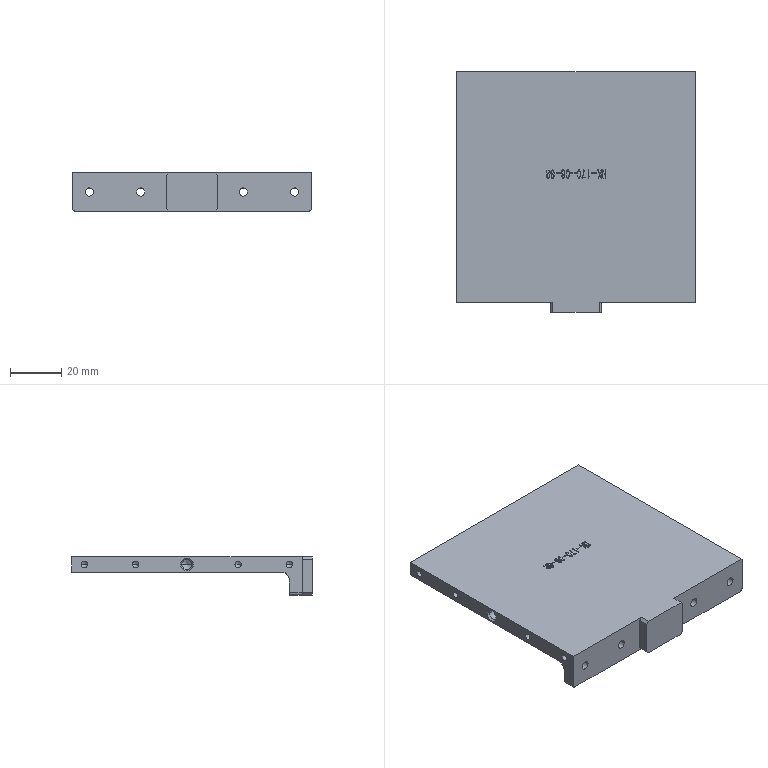NC program | NX | posted with a generic post | part box 93.2 x 94 x 15 mm
Lines 1 to 888 of 2664:
N10 G17 G21 G94 G90
(ZLEVEL_PROFILE_COPY_1_COPY , TOOL : D10)
N12 T15 M6
N14 G54
N16 G17 G0 G90 X-14.89 Y-48.506 B0. C0. S9500 M3
N18 G43 Z30. H15
N20 Z1.5
N22 G94 G1 X-14.98 Y-48.1 Z1.478 F1000.
N24 X-47.154 Z-0.208
N26 X-48.498 Y-47.766 Z-0.281
N28 X-49.704 Y-47.084 Z-0.353
N30 X-50.684 Y-46.104 Z-0.426
N32 X-51.366 Y-44.898 Z-0.498
N34 X-51.7 Y-43.554 Z-0.571
N36 Y-43. Z-0.6
N38 Y47. F3000.
N40 G2 X-46.6 Y52.1 R5.1
N42 G1 X46.6
N44 G2 X51.7 Y47. R5.1
N46 G1 Y-43.
N48 G2 X46.6 Y-48.1 R5.1
N50 G1 X14.98
N52 G2 X10. Y-52.1 R5.1
N54 G1 X-10.
N56 G2 X-14.98 Y-48.1 R5.1
N58 G1 X-46.6
N60 G2 X-51.7 Y-43. R5.1
N62 G1 Y47. Z-0.734
N64 X-51.675 Y47.5 Z-0.735
N66 X-51.602 Y47.995 Z-0.736
N68 X-51.48 Y48.48
N70 X-51.312 Y48.952 Z-0.737
N72 X-51.098 Y49.404 Z-0.738
N74 X-50.84 Y49.833 Z-0.739
N76 X-50.542 Y50.235
N78 X-50.206 Y50.606 Z-0.74
N80 X-49.835 Y50.942 Z-0.741
N82 X-49.433 Y51.24 Z-0.742
N84 X-49.004 Y51.498
N86 X-48.552 Y51.712 Z-0.743
N88 X-48.08 Y51.88 Z-0.744
N90 X-47.595 Y52.002 Z-0.745
N92 X-47.1 Y52.075
N94 X-46.6 Y52.1 Z-0.746
N96 X46.6 Z-0.885
N98 X47.1 Y52.075 Z-0.886
N100 X47.595 Y52.002 Z-0.887
N102 X48.08 Y51.88
N104 X48.552 Y51.712 Z-0.888
N106 X49.004 Y51.498 Z-0.889
N108 X49.433 Y51.24 Z-0.89
N110 X49.835 Y50.942
N112 X50.206 Y50.606 Z-0.891
N114 X50.542 Y50.235 Z-0.892
N116 X50.84 Y49.833 Z-0.893
N118 X51.098 Y49.404
N120 X51.312 Y48.952 Z-0.894
N122 X51.48 Y48.48 Z-0.895
N124 X51.602 Y47.995 Z-0.896
N126 X51.675 Y47.5
N128 X51.7 Y47. Z-0.897
N130 Y-43. Z-1.031
N132 X51.675 Y-43.5 Z-1.032
N134 X51.602 Y-43.995 Z-1.033
N136 X51.48 Y-44.48 Z-1.034
N138 X51.312 Y-44.952
N140 X51.098 Y-45.404 Z-1.035
N142 X50.84 Y-45.833 Z-1.036
N144 X50.542 Y-46.235 Z-1.037
N146 X50.206 Y-46.606
N148 X49.835 Y-46.942 Z-1.038
N150 X49.433 Y-47.24 Z-1.039
N152 X49.004 Y-47.498 Z-1.04
N154 X48.552 Y-47.712
N156 X48.08 Y-47.88 Z-1.041
N158 X47.595 Y-48.002 Z-1.042
N160 X47.1 Y-48.075 Z-1.043
N162 X46.6 Y-48.1
N164 X14.98 Z-1.091
N166 X14.848 Y-48.584
N168 X14.676 Y-49.036 Z-1.092
N170 X14.457 Y-49.478 Z-1.093
N172 X14.197 Y-49.897
N174 X13.898 Y-50.288 Z-1.094
N176 X13.563 Y-50.649 Z-1.095
N178 X13.194 Y-50.976 Z-1.096
N180 X12.795 Y-51.266
N182 X12.37 Y-51.516 Z-1.097
N184 X11.923 Y-51.723 Z-1.098
N186 X11.458 Y-51.887 Z-1.099
N188 X10.98 Y-52.005
N190 X10.492 Y-52.076 Z-1.1
N192 X10. Y-52.1 Z-1.101
N194 X-10. Z-1.131
N196 X-10.492 Y-52.076
N198 X-10.98 Y-52.005 Z-1.132
N200 X-11.458 Y-51.887 Z-1.133
N202 X-11.923 Y-51.723 Z-1.134
N204 X-12.37 Y-51.516
N206 X-12.795 Y-51.266 Z-1.135
N208 X-13.194 Y-50.976 Z-1.136
N210 X-13.563 Y-50.649
N212 X-13.898 Y-50.288 Z-1.137
N214 X-14.197 Y-49.897 Z-1.138
N216 X-14.457 Y-49.478 Z-1.139
N218 X-14.676 Y-49.036
N220 X-14.848 Y-48.584 Z-1.14
N222 X-14.98 Y-48.1 Z-1.141
N224 X-46.6 Z-1.188
N226 X-47.1 Y-48.075 Z-1.189
N228 X-47.595 Y-48.002 Z-1.19
N230 X-48.08 Y-47.88
N232 X-48.552 Y-47.712 Z-1.191
N234 X-49.004 Y-47.498 Z-1.192
N236 X-49.433 Y-47.24 Z-1.193
N238 X-49.835 Y-46.942
N240 X-50.206 Y-46.606 Z-1.194
N242 X-50.542 Y-46.235 Z-1.195
N244 X-50.84 Y-45.833 Z-1.196
N246 X-51.098 Y-45.404
N248 X-51.312 Y-44.952 Z-1.197
N250 X-51.48 Y-44.48 Z-1.198
N252 X-51.602 Y-43.995 Z-1.199
N254 X-51.675 Y-43.5
N256 X-51.7 Y-43. Z-1.2
N258 Y47. Z-1.334
N260 X-51.675 Y47.5 Z-1.335
N262 X-51.602 Y47.995 Z-1.336
N264 X-51.48 Y48.48
N266 X-51.312 Y48.952 Z-1.337
N268 X-51.098 Y49.404 Z-1.338
N270 X-50.84 Y49.833 Z-1.339
N272 X-50.542 Y50.235
N274 X-50.206 Y50.606 Z-1.34
N276 X-49.835 Y50.942 Z-1.341
N278 X-49.433 Y51.24 Z-1.342
N280 X-49.004 Y51.498
N282 X-48.552 Y51.712 Z-1.343
N284 X-48.08 Y51.88 Z-1.344
N286 X-47.595 Y52.002 Z-1.345
N288 X-47.1 Y52.075
N290 X-46.6 Y52.1 Z-1.346
N292 X46.6 Z-1.485
N294 X47.1 Y52.075 Z-1.486
N296 X47.595 Y52.002 Z-1.487
N298 X48.08 Y51.88
N300 X48.552 Y51.712 Z-1.488
N302 X49.004 Y51.498 Z-1.489
N304 X49.433 Y51.24 Z-1.49
N306 X49.835 Y50.942
N308 X50.206 Y50.606 Z-1.491
N310 X50.542 Y50.235 Z-1.492
N312 X50.84 Y49.833 Z-1.493
N314 X51.098 Y49.404
N316 X51.312 Y48.952 Z-1.494
N318 X51.48 Y48.48 Z-1.495
N320 X51.602 Y47.995 Z-1.496
N322 X51.675 Y47.5
N324 X51.7 Y47. Z-1.497
N326 Y-43. Z-1.631
N328 X51.675 Y-43.5 Z-1.632
N330 X51.602 Y-43.995 Z-1.633
N332 X51.48 Y-44.48 Z-1.634
N334 X51.312 Y-44.952
N336 X51.098 Y-45.404 Z-1.635
N338 X50.84 Y-45.833 Z-1.636
N340 X50.542 Y-46.235 Z-1.637
N342 X50.206 Y-46.606
N344 X49.835 Y-46.942 Z-1.638
N346 X49.433 Y-47.24 Z-1.639
N348 X49.004 Y-47.498 Z-1.64
N350 X48.552 Y-47.712
N352 X48.08 Y-47.88 Z-1.641
N354 X47.595 Y-48.002 Z-1.642
N356 X47.1 Y-48.075 Z-1.643
N358 X46.6 Y-48.1
N360 X14.98 Z-1.691
N362 X14.848 Y-48.584
N364 X14.676 Y-49.036 Z-1.692
N366 X14.457 Y-49.478 Z-1.693
N368 X14.197 Y-49.897
N370 X13.898 Y-50.288 Z-1.694
N372 X13.563 Y-50.649 Z-1.695
N374 X13.194 Y-50.976 Z-1.696
N376 X12.795 Y-51.266
N378 X12.37 Y-51.516 Z-1.697
N380 X11.923 Y-51.723 Z-1.698
N382 X11.458 Y-51.887 Z-1.699
N384 X10.98 Y-52.005
N386 X10.492 Y-52.076 Z-1.7
N388 X10. Y-52.1 Z-1.701
N390 X-10. Z-1.731
N392 X-10.492 Y-52.076
N394 X-10.98 Y-52.005 Z-1.732
N396 X-11.458 Y-51.887 Z-1.733
N398 X-11.923 Y-51.723 Z-1.734
N400 X-12.37 Y-51.516
N402 X-12.795 Y-51.266 Z-1.735
N404 X-13.194 Y-50.976 Z-1.736
N406 X-13.563 Y-50.649
N408 X-13.898 Y-50.288 Z-1.737
N410 X-14.197 Y-49.897 Z-1.738
N412 X-14.457 Y-49.478 Z-1.739
N414 X-14.676 Y-49.036
N416 X-14.848 Y-48.584 Z-1.74
N418 X-14.98 Y-48.1 Z-1.741
N420 X-46.6 Z-1.788
N422 X-47.1 Y-48.075 Z-1.789
N424 X-47.595 Y-48.002 Z-1.79
N426 X-48.08 Y-47.88
N428 X-48.552 Y-47.712 Z-1.791
N430 X-49.004 Y-47.498 Z-1.792
N432 X-49.433 Y-47.24 Z-1.793
N434 X-49.835 Y-46.942
N436 X-50.206 Y-46.606 Z-1.794
N438 X-50.542 Y-46.235 Z-1.795
N440 X-50.84 Y-45.833 Z-1.796
N442 X-51.098 Y-45.404
N444 X-51.312 Y-44.952 Z-1.797
N446 X-51.48 Y-44.48 Z-1.798
N448 X-51.602 Y-43.995 Z-1.799
N450 X-51.675 Y-43.5
N452 X-51.7 Y-43. Z-1.8
N454 Y47. Z-1.934
N456 X-51.675 Y47.5 Z-1.935
N458 X-51.602 Y47.995 Z-1.936
N460 X-51.48 Y48.48
N462 X-51.312 Y48.952 Z-1.937
N464 X-51.098 Y49.404 Z-1.938
N466 X-50.84 Y49.833 Z-1.939
N468 X-50.542 Y50.235
N470 X-50.206 Y50.606 Z-1.94
N472 X-49.835 Y50.942 Z-1.941
N474 X-49.433 Y51.24 Z-1.942
N476 X-49.004 Y51.498
N478 X-48.552 Y51.712 Z-1.943
N480 X-48.08 Y51.88 Z-1.944
N482 X-47.595 Y52.002 Z-1.945
N484 X-47.1 Y52.075
N486 X-46.6 Y52.1 Z-1.946
N488 X46.6 Z-2.085
N490 X47.1 Y52.075 Z-2.086
N492 X47.595 Y52.002 Z-2.087
N494 X48.08 Y51.88
N496 X48.552 Y51.712 Z-2.088
N498 X49.004 Y51.498 Z-2.089
N500 X49.433 Y51.24 Z-2.09
N502 X49.835 Y50.942
N504 X50.206 Y50.606 Z-2.091
N506 X50.542 Y50.235 Z-2.092
N508 X50.84 Y49.833 Z-2.093
N510 X51.098 Y49.404
N512 X51.312 Y48.952 Z-2.094
N514 X51.48 Y48.48 Z-2.095
N516 X51.602 Y47.995 Z-2.096
N518 X51.675 Y47.5
N520 X51.7 Y47. Z-2.097
N522 Y-43. Z-2.231
N524 X51.675 Y-43.5 Z-2.232
N526 X51.602 Y-43.995 Z-2.233
N528 X51.48 Y-44.48 Z-2.234
N530 X51.312 Y-44.952
N532 X51.098 Y-45.404 Z-2.235
N534 X50.84 Y-45.833 Z-2.236
N536 X50.542 Y-46.235 Z-2.237
N538 X50.206 Y-46.606
N540 X49.835 Y-46.942 Z-2.238
N542 X49.433 Y-47.24 Z-2.239
N544 X49.004 Y-47.498 Z-2.24
N546 X48.552 Y-47.712
N548 X48.08 Y-47.88 Z-2.241
N550 X47.595 Y-48.002 Z-2.242
N552 X47.1 Y-48.075 Z-2.243
N554 X46.6 Y-48.1
N556 X14.98 Z-2.291
N558 X14.848 Y-48.584
N560 X14.676 Y-49.036 Z-2.292
N562 X14.457 Y-49.478 Z-2.293
N564 X14.197 Y-49.897
N566 X13.898 Y-50.288 Z-2.294
N568 X13.563 Y-50.649 Z-2.295
N570 X13.194 Y-50.976 Z-2.296
N572 X12.795 Y-51.266
N574 X12.37 Y-51.516 Z-2.297
N576 X11.923 Y-51.723 Z-2.298
N578 X11.458 Y-51.887 Z-2.299
N580 X10.98 Y-52.005
N582 X10.492 Y-52.076 Z-2.3
N584 X10. Y-52.1 Z-2.301
N586 X-10. Z-2.331
N588 X-10.492 Y-52.076
N590 X-10.98 Y-52.005 Z-2.332
N592 X-11.458 Y-51.887 Z-2.333
N594 X-11.923 Y-51.723 Z-2.334
N596 X-12.37 Y-51.516
N598 X-12.795 Y-51.266 Z-2.335
N600 X-13.194 Y-50.976 Z-2.336
N602 X-13.563 Y-50.649
N604 X-13.898 Y-50.288 Z-2.337
N606 X-14.197 Y-49.897 Z-2.338
N608 X-14.457 Y-49.478 Z-2.339
N610 X-14.676 Y-49.036
N612 X-14.848 Y-48.584 Z-2.34
N614 X-14.98 Y-48.1 Z-2.341
N616 X-46.6 Z-2.388
N618 X-47.1 Y-48.075 Z-2.389
N620 X-47.595 Y-48.002 Z-2.39
N622 X-48.08 Y-47.88
N624 X-48.552 Y-47.712 Z-2.391
N626 X-49.004 Y-47.498 Z-2.392
N628 X-49.433 Y-47.24 Z-2.393
N630 X-49.835 Y-46.942
N632 X-50.206 Y-46.606 Z-2.394
N634 X-50.542 Y-46.235 Z-2.395
N636 X-50.84 Y-45.833 Z-2.396
N638 X-51.098 Y-45.404
N640 X-51.312 Y-44.952 Z-2.397
N642 X-51.48 Y-44.48 Z-2.398
N644 X-51.602 Y-43.995 Z-2.399
N646 X-51.675 Y-43.5
N648 X-51.7 Y-43. Z-2.4
N650 Y47. Z-2.534
N652 X-51.675 Y47.5 Z-2.535
N654 X-51.602 Y47.995 Z-2.536
N656 X-51.48 Y48.48
N658 X-51.312 Y48.952 Z-2.537
N660 X-51.098 Y49.404 Z-2.538
N662 X-50.84 Y49.833 Z-2.539
N664 X-50.542 Y50.235
N666 X-50.206 Y50.606 Z-2.54
N668 X-49.835 Y50.942 Z-2.541
N670 X-49.433 Y51.24 Z-2.542
N672 X-49.004 Y51.498
N674 X-48.552 Y51.712 Z-2.543
N676 X-48.08 Y51.88 Z-2.544
N678 X-47.595 Y52.002 Z-2.545
N680 X-47.1 Y52.075
N682 X-46.6 Y52.1 Z-2.546
N684 X46.6 Z-2.685
N686 X47.1 Y52.075 Z-2.686
N688 X47.595 Y52.002 Z-2.687
N690 X48.08 Y51.88
N692 X48.552 Y51.712 Z-2.688
N694 X49.004 Y51.498 Z-2.689
N696 X49.433 Y51.24 Z-2.69
N698 X49.835 Y50.942
N700 X50.206 Y50.606 Z-2.691
N702 X50.542 Y50.235 Z-2.692
N704 X50.84 Y49.833 Z-2.693
N706 X51.098 Y49.404
N708 X51.312 Y48.952 Z-2.694
N710 X51.48 Y48.48 Z-2.695
N712 X51.602 Y47.995 Z-2.696
N714 X51.675 Y47.5
N716 X51.7 Y47. Z-2.697
N718 Y-43. Z-2.831
N720 X51.675 Y-43.5 Z-2.832
N722 X51.602 Y-43.995 Z-2.833
N724 X51.48 Y-44.48 Z-2.834
N726 X51.312 Y-44.952
N728 X51.098 Y-45.404 Z-2.835
N730 X50.84 Y-45.833 Z-2.836
N732 X50.542 Y-46.235 Z-2.837
N734 X50.206 Y-46.606
N736 X49.835 Y-46.942 Z-2.838
N738 X49.433 Y-47.24 Z-2.839
N740 X49.004 Y-47.498 Z-2.84
N742 X48.552 Y-47.712
N744 X48.08 Y-47.88 Z-2.841
N746 X47.595 Y-48.002 Z-2.842
N748 X47.1 Y-48.075 Z-2.843
N750 X46.6 Y-48.1
N752 X14.98 Z-2.891
N754 X14.848 Y-48.584
N756 X14.676 Y-49.036 Z-2.892
N758 X14.457 Y-49.478 Z-2.893
N760 X14.197 Y-49.897
N762 X13.898 Y-50.288 Z-2.894
N764 X13.563 Y-50.649 Z-2.895
N766 X13.194 Y-50.976 Z-2.896
N768 X12.795 Y-51.266
N770 X12.37 Y-51.516 Z-2.897
N772 X11.923 Y-51.723 Z-2.898
N774 X11.458 Y-51.887 Z-2.899
N776 X10.98 Y-52.005
N778 X10.492 Y-52.076 Z-2.9
N780 X10. Y-52.1 Z-2.901
N782 X-10. Z-2.931
N784 X-10.492 Y-52.076
N786 X-10.98 Y-52.005 Z-2.932
N788 X-11.458 Y-51.887 Z-2.933
N790 X-11.923 Y-51.723 Z-2.934
N792 X-12.37 Y-51.516
N794 X-12.795 Y-51.266 Z-2.935
N796 X-13.194 Y-50.976 Z-2.936
N798 X-13.563 Y-50.649
N800 X-13.898 Y-50.288 Z-2.937
N802 X-14.197 Y-49.897 Z-2.938
N804 X-14.457 Y-49.478 Z-2.939
N806 X-14.676 Y-49.036
N808 X-14.848 Y-48.584 Z-2.94
N810 X-14.98 Y-48.1 Z-2.941
N812 X-46.6 Z-2.988
N814 X-47.1 Y-48.075 Z-2.989
N816 X-47.595 Y-48.002 Z-2.99
N818 X-48.08 Y-47.88
N820 X-48.552 Y-47.712 Z-2.991
N822 X-49.004 Y-47.498 Z-2.992
N824 X-49.433 Y-47.24 Z-2.993
N826 X-49.835 Y-46.942
N828 X-50.206 Y-46.606 Z-2.994
N830 X-50.542 Y-46.235 Z-2.995
N832 X-50.84 Y-45.833 Z-2.996
N834 X-51.098 Y-45.404
N836 X-51.312 Y-44.952 Z-2.997
N838 X-51.48 Y-44.48 Z-2.998
N840 X-51.602 Y-43.995 Z-2.999
N842 X-51.675 Y-43.5
N844 X-51.7 Y-43. Z-3.
N846 Y47. Z-3.134
N848 X-51.675 Y47.5 Z-3.135
N850 X-51.602 Y47.995 Z-3.136
N852 X-51.48 Y48.48
N854 X-51.312 Y48.952 Z-3.137
N856 X-51.098 Y49.404 Z-3.138
N858 X-50.84 Y49.833 Z-3.139
N860 X-50.542 Y50.235
N862 X-50.206 Y50.606 Z-3.14
N864 X-49.835 Y50.942 Z-3.141
N866 X-49.433 Y51.24 Z-3.142
N868 X-49.004 Y51.498
N870 X-48.552 Y51.712 Z-3.143
N872 X-48.08 Y51.88 Z-3.144
N874 X-47.595 Y52.002 Z-3.145
N876 X-47.1 Y52.075
N878 X-46.6 Y52.1 Z-3.146
N880 X46.6 Z-3.285
N882 X47.1 Y52.075 Z-3.286
N884 X47.595 Y52.002 Z-3.287
N886 X48.08 Y51.88
N888 X48.552 Y51.712 Z-3.288
N890 X49.004 Y51.498 Z-3.289
N892 X49.433 Y51.24 Z-3.29
N894 X49.835 Y50.942
N896 X50.206 Y50.606 Z-3.291
N898 X50.542 Y50.235 Z-3.292
N900 X50.84 Y49.833 Z-3.293
N902 X51.098 Y49.404
N904 X51.312 Y48.952 Z-3.294
N906 X51.48 Y48.48 Z-3.295
N908 X51.602 Y47.995 Z-3.296
N910 X51.675 Y47.5
N912 X51.7 Y47. Z-3.297
N914 Y-43. Z-3.431
N916 X51.675 Y-43.5 Z-3.432
N918 X51.602 Y-43.995 Z-3.433
N920 X51.48 Y-44.48 Z-3.434
N922 X51.312 Y-44.952
N924 X51.098 Y-45.404 Z-3.435
N926 X50.84 Y-45.833 Z-3.436
N928 X50.542 Y-46.235 Z-3.437
N930 X50.206 Y-46.606
N932 X49.835 Y-46.942 Z-3.438
N934 X49.433 Y-47.24 Z-3.439
N936 X49.004 Y-47.498 Z-3.44
N938 X48.552 Y-47.712
N940 X48.08 Y-47.88 Z-3.441
N942 X47.595 Y-48.002 Z-3.442
N944 X47.1 Y-48.075 Z-3.443
N946 X46.6 Y-48.1
N948 X14.98 Z-3.491
N950 X14.848 Y-48.584
N952 X14.676 Y-49.036 Z-3.492
N954 X14.457 Y-49.478 Z-3.493
N956 X14.197 Y-49.897
N958 X13.898 Y-50.288 Z-3.494
N960 X13.563 Y-50.649 Z-3.495
N962 X13.194 Y-50.976 Z-3.496
N964 X12.795 Y-51.266
N966 X12.37 Y-51.516 Z-3.497
N968 X11.923 Y-51.723 Z-3.498
N970 X11.458 Y-51.887 Z-3.499
N972 X10.98 Y-52.005
N974 X10.492 Y-52.076 Z-3.5
N976 X10. Y-52.1 Z-3.501
N978 X-10. Z-3.531
N980 X-10.492 Y-52.076
N982 X-10.98 Y-52.005 Z-3.532
N984 X-11.458 Y-51.887 Z-3.533
N986 X-11.923 Y-51.723 Z-3.534
N988 X-12.37 Y-51.516
N990 X-12.795 Y-51.266 Z-3.535
N992 X-13.194 Y-50.976 Z-3.536
N994 X-13.563 Y-50.649
N996 X-13.898 Y-50.288 Z-3.537
N998 X-14.197 Y-49.897 Z-3.538
N1000 X-14.457 Y-49.478 Z-3.539
N1002 X-14.676 Y-49.036
N1004 X-14.848 Y-48.584 Z-3.54
N1006 X-14.98 Y-48.1 Z-3.541
N1008 X-46.6 Z-3.588
N1010 X-47.1 Y-48.075 Z-3.589
N1012 X-47.595 Y-48.002 Z-3.59
N1014 X-48.08 Y-47.88
N1016 X-48.552 Y-47.712 Z-3.591
N1018 X-49.004 Y-47.498 Z-3.592
N1020 X-49.433 Y-47.24 Z-3.593
N1022 X-49.835 Y-46.942
N1024 X-50.206 Y-46.606 Z-3.594
N1026 X-50.542 Y-46.235 Z-3.595
N1028 X-50.84 Y-45.833 Z-3.596
N1030 X-51.098 Y-45.404
N1032 X-51.312 Y-44.952 Z-3.597
N1034 X-51.48 Y-44.48 Z-3.598
N1036 X-51.602 Y-43.995 Z-3.599
N1038 X-51.675 Y-43.5
N1040 X-51.7 Y-43. Z-3.6
N1042 Y47. Z-3.734
N1044 X-51.675 Y47.5 Z-3.735
N1046 X-51.602 Y47.995 Z-3.736
N1048 X-51.48 Y48.48
N1050 X-51.312 Y48.952 Z-3.737
N1052 X-51.098 Y49.404 Z-3.738
N1054 X-50.84 Y49.833 Z-3.739
N1056 X-50.542 Y50.235
N1058 X-50.206 Y50.606 Z-3.74
N1060 X-49.835 Y50.942 Z-3.741
N1062 X-49.433 Y51.24 Z-3.742
N1064 X-49.004 Y51.498
N1066 X-48.552 Y51.712 Z-3.743
N1068 X-48.08 Y51.88 Z-3.744
N1070 X-47.595 Y52.002 Z-3.745
N1072 X-47.1 Y52.075
N1074 X-46.6 Y52.1 Z-3.746
N1076 X46.6 Z-3.885
N1078 X47.1 Y52.075 Z-3.886
N1080 X47.595 Y52.002 Z-3.887
N1082 X48.08 Y51.88
N1084 X48.552 Y51.712 Z-3.888
N1086 X49.004 Y51.498 Z-3.889
N1088 X49.433 Y51.24 Z-3.89
N1090 X49.835 Y50.942
N1092 X50.206 Y50.606 Z-3.891
N1094 X50.542 Y50.235 Z-3.892
N1096 X50.84 Y49.833 Z-3.893
N1098 X51.098 Y49.404
N1100 X51.312 Y48.952 Z-3.894
N1102 X51.48 Y48.48 Z-3.895
N1104 X51.602 Y47.995 Z-3.896
N1106 X51.675 Y47.5
N1108 X51.7 Y47. Z-3.897
N1110 Y-43. Z-4.031
N1112 X51.675 Y-43.5 Z-4.032
N1114 X51.602 Y-43.995 Z-4.033
N1116 X51.48 Y-44.48 Z-4.034
N1118 X51.312 Y-44.952
N1120 X51.098 Y-45.404 Z-4.035
N1122 X50.84 Y-45.833 Z-4.036
N1124 X50.542 Y-46.235 Z-4.037
N1126 X50.206 Y-46.606
N1128 X49.835 Y-46.942 Z-4.038
N1130 X49.433 Y-47.24 Z-4.039
N1132 X49.004 Y-47.498 Z-4.04
N1134 X48.552 Y-47.712
N1136 X48.08 Y-47.88 Z-4.041
N1138 X47.595 Y-48.002 Z-4.042
N1140 X47.1 Y-48.075 Z-4.043
N1142 X46.6 Y-48.1
N1144 X14.98 Z-4.091
N1146 X14.848 Y-48.584
N1148 X14.676 Y-49.036 Z-4.092
N1150 X14.457 Y-49.478 Z-4.093
N1152 X14.197 Y-49.897
N1154 X13.898 Y-50.288 Z-4.094
N1156 X13.563 Y-50.649 Z-4.095
N1158 X13.194 Y-50.976 Z-4.096
N1160 X12.795 Y-51.266
N1162 X12.37 Y-51.516 Z-4.097
N1164 X11.923 Y-51.723 Z-4.098
N1166 X11.458 Y-51.887 Z-4.099
N1168 X10.98 Y-52.005
N1170 X10.492 Y-52.076 Z-4.1
N1172 X10. Y-52.1 Z-4.101
N1174 X-10. Z-4.131
N1176 X-10.492 Y-52.076
N1178 X-10.98 Y-52.005 Z-4.132
N1180 X-11.458 Y-51.887 Z-4.133
N1182 X-11.923 Y-51.723 Z-4.134
N1184 X-12.37 Y-51.516
N1186 X-12.795 Y-51.266 Z-4.135
N1188 X-13.194 Y-50.976 Z-4.136
N1190 X-13.563 Y-50.649
N1192 X-13.898 Y-50.288 Z-4.137
N1194 X-14.197 Y-49.897 Z-4.138
N1196 X-14.457 Y-49.478 Z-4.139
N1198 X-14.676 Y-49.036
N1200 X-14.848 Y-48.584 Z-4.14
N1202 X-14.98 Y-48.1 Z-4.141
N1204 X-46.6 Z-4.188
N1206 X-47.1 Y-48.075 Z-4.189
N1208 X-47.595 Y-48.002 Z-4.19
N1210 X-48.08 Y-47.88
N1212 X-48.552 Y-47.712 Z-4.191
N1214 X-49.004 Y-47.498 Z-4.192
N1216 X-49.433 Y-47.24 Z-4.193
N1218 X-49.835 Y-46.942
N1220 X-50.206 Y-46.606 Z-4.194
N1222 X-50.542 Y-46.235 Z-4.195
N1224 X-50.84 Y-45.833 Z-4.196
N1226 X-51.098 Y-45.404
N1228 X-51.312 Y-44.952 Z-4.197
N1230 X-51.48 Y-44.48 Z-4.198
N1232 X-51.602 Y-43.995 Z-4.199
N1234 X-51.675 Y-43.5
N1236 X-51.7 Y-43. Z-4.2
N1238 Y47. Z-4.334
N1240 X-51.675 Y47.5 Z-4.335
N1242 X-51.602 Y47.995 Z-4.336
N1244 X-51.48 Y48.48
N1246 X-51.312 Y48.952 Z-4.337
N1248 X-51.098 Y49.404 Z-4.338
N1250 X-50.84 Y49.833 Z-4.339
N1252 X-50.542 Y50.235
N1254 X-50.206 Y50.606 Z-4.34
N1256 X-49.835 Y50.942 Z-4.341
N1258 X-49.433 Y51.24 Z-4.342
N1260 X-49.004 Y51.498
N1262 X-48.552 Y51.712 Z-4.343
N1264 X-48.08 Y51.88 Z-4.344
N1266 X-47.595 Y52.002 Z-4.345
N1268 X-47.1 Y52.075
N1270 X-46.6 Y52.1 Z-4.346
N1272 X46.6 Z-4.485
N1274 X47.1 Y52.075 Z-4.486
N1276 X47.595 Y52.002 Z-4.487
N1278 X48.08 Y51.88
N1280 X48.552 Y51.712 Z-4.488
N1282 X49.004 Y51.498 Z-4.489
N1284 X49.433 Y51.24 Z-4.49
N1286 X49.835 Y50.942
N1288 X50.206 Y50.606 Z-4.491
N1290 X50.542 Y50.235 Z-4.492
N1292 X50.84 Y49.833 Z-4.493
N1294 X51.098 Y49.404
N1296 X51.312 Y48.952 Z-4.494
N1298 X51.48 Y48.48 Z-4.495
N1300 X51.602 Y47.995 Z-4.496
N1302 X51.675 Y47.5
N1304 X51.7 Y47. Z-4.497
N1306 Y-43. Z-4.631
N1308 X51.675 Y-43.5 Z-4.632
N1310 X51.602 Y-43.995 Z-4.633
N1312 X51.48 Y-44.48 Z-4.634
N1314 X51.312 Y-44.952
N1316 X51.098 Y-45.404 Z-4.635
N1318 X50.84 Y-45.833 Z-4.636
N1320 X50.542 Y-46.235 Z-4.637
N1322 X50.206 Y-46.606
N1324 X49.835 Y-46.942 Z-4.638
N1326 X49.433 Y-47.24 Z-4.639
N1328 X49.004 Y-47.498 Z-4.64
N1330 X48.552 Y-47.712
N1332 X48.08 Y-47.88 Z-4.641
N1334 X47.595 Y-48.002 Z-4.642
N1336 X47.1 Y-48.075 Z-4.643
N1338 X46.6 Y-48.1
N1340 X14.98 Z-4.691
N1342 X14.848 Y-48.584
N1344 X14.676 Y-49.036 Z-4.692
N1346 X14.457 Y-49.478 Z-4.693
N1348 X14.197 Y-49.897
N1350 X13.898 Y-50.288 Z-4.694
N1352 X13.563 Y-50.649 Z-4.695
N1354 X13.194 Y-50.976 Z-4.696
N1356 X12.795 Y-51.266
N1358 X12.37 Y-51.516 Z-4.697
N1360 X11.923 Y-51.723 Z-4.698
N1362 X11.458 Y-51.887 Z-4.699
N1364 X10.98 Y-52.005
N1366 X10.492 Y-52.076 Z-4.7
N1368 X10. Y-52.1 Z-4.701
N1370 X-10. Z-4.731
N1372 X-10.492 Y-52.076
N1374 X-10.98 Y-52.005 Z-4.732
N1376 X-11.458 Y-51.887 Z-4.733
N1378 X-11.923 Y-51.723 Z-4.734
N1380 X-12.37 Y-51.516
N1382 X-12.795 Y-51.266 Z-4.735
N1384 X-13.194 Y-50.976 Z-4.736
N1386 X-13.563 Y-50.649
N1388 X-13.898 Y-50.288 Z-4.737
N1390 X-14.197 Y-49.897 Z-4.738
N1392 X-14.457 Y-49.478 Z-4.739
N1394 X-14.676 Y-49.036
N1396 X-14.848 Y-48.584 Z-4.74
N1398 X-14.98 Y-48.1 Z-4.741
N1400 X-46.6 Z-4.788
N1402 X-47.1 Y-48.075 Z-4.789
N1404 X-47.595 Y-48.002 Z-4.79
N1406 X-48.08 Y-47.88
N1408 X-48.552 Y-47.712 Z-4.791
N1410 X-49.004 Y-47.498 Z-4.792
N1412 X-49.433 Y-47.24 Z-4.793
N1414 X-49.835 Y-46.942
N1416 X-50.206 Y-46.606 Z-4.794
N1418 X-50.542 Y-46.235 Z-4.795
N1420 X-50.84 Y-45.833 Z-4.796
N1422 X-51.098 Y-45.404
N1424 X-51.312 Y-44.952 Z-4.797
N1426 X-51.48 Y-44.48 Z-4.798
N1428 X-51.602 Y-43.995 Z-4.799
N1430 X-51.675 Y-43.5
N1432 X-51.7 Y-43. Z-4.8
N1434 Y47. Z-4.934
N1436 X-51.675 Y47.5 Z-4.935
N1438 X-51.602 Y47.995 Z-4.936
N1440 X-51.48 Y48.48
N1442 X-51.312 Y48.952 Z-4.937
N1444 X-51.098 Y49.404 Z-4.938
N1446 X-50.84 Y49.833 Z-4.939
N1448 X-50.542 Y50.235
N1450 X-50.206 Y50.606 Z-4.94
N1452 X-49.835 Y50.942 Z-4.941
N1454 X-49.433 Y51.24 Z-4.942
N1456 X-49.004 Y51.498
N1458 X-48.552 Y51.712 Z-4.943
N1460 X-48.08 Y51.88 Z-4.944
N1462 X-47.595 Y52.002 Z-4.945
N1464 X-47.1 Y52.075
N1466 X-46.6 Y52.1 Z-4.946
N1468 X46.6 Z-5.085
N1470 X47.1 Y52.075 Z-5.086
N1472 X47.595 Y52.002 Z-5.087
N1474 X48.08 Y51.88
N1476 X48.552 Y51.712 Z-5.088
N1478 X49.004 Y51.498 Z-5.089
N1480 X49.433 Y51.24 Z-5.09
N1482 X49.835 Y50.942
N1484 X50.206 Y50.606 Z-5.091
N1486 X50.542 Y50.235 Z-5.092
N1488 X50.84 Y49.833 Z-5.093
N1490 X51.098 Y49.404
N1492 X51.312 Y48.952 Z-5.094
N1494 X51.48 Y48.48 Z-5.095
N1496 X51.602 Y47.995 Z-5.096
N1498 X51.675 Y47.5
N1500 X51.7 Y47. Z-5.097
N1502 Y-43. Z-5.231
N1504 X51.675 Y-43.5 Z-5.232
N1506 X51.602 Y-43.995 Z-5.233
N1508 X51.48 Y-44.48 Z-5.234
N1510 X51.312 Y-44.952
N1512 X51.098 Y-45.404 Z-5.235
N1514 X50.84 Y-45.833 Z-5.236
N1516 X50.542 Y-46.235 Z-5.237
N1518 X50.206 Y-46.606
N1520 X49.835 Y-46.942 Z-5.238
N1522 X49.433 Y-47.24 Z-5.239
N1524 X49.004 Y-47.498 Z-5.24
N1526 X48.552 Y-47.712
N1528 X48.08 Y-47.88 Z-5.241
N1530 X47.595 Y-48.002 Z-5.242
N1532 X47.1 Y-48.075 Z-5.243
N1534 X46.6 Y-48.1
N1536 X14.98 Z-5.291
N1538 X14.848 Y-48.584
N1540 X14.676 Y-49.036 Z-5.292
N1542 X14.457 Y-49.478 Z-5.293
N1544 X14.197 Y-49.897
N1546 X13.898 Y-50.288 Z-5.294
N1548 X13.563 Y-50.649 Z-5.295
N1550 X13.194 Y-50.976 Z-5.296
N1552 X12.795 Y-51.266
N1554 X12.37 Y-51.516 Z-5.297
N1556 X11.923 Y-51.723 Z-5.298
N1558 X11.458 Y-51.887 Z-5.299
N1560 X10.98 Y-52.005
N1562 X10.492 Y-52.076 Z-5.3
N1564 X10. Y-52.1 Z-5.301
N1566 X-10. Z-5.331
N1568 X-10.492 Y-52.076
N1570 X-10.98 Y-52.005 Z-5.332
N1572 X-11.458 Y-51.887 Z-5.333
N1574 X-11.923 Y-51.723 Z-5.334
N1576 X-12.37 Y-51.516
N1578 X-12.795 Y-51.266 Z-5.335
N1580 X-13.194 Y-50.976 Z-5.336
N1582 X-13.563 Y-50.649
N1584 X-13.898 Y-50.288 Z-5.337
N1586 X-14.197 Y-49.897 Z-5.338
N1588 X-14.457 Y-49.478 Z-5.339
N1590 X-14.676 Y-49.036
N1592 X-14.848 Y-48.584 Z-5.34
N1594 X-14.98 Y-48.1 Z-5.341
N1596 X-46.6 Z-5.388
N1598 X-47.1 Y-48.075 Z-5.389
N1600 X-47.595 Y-48.002 Z-5.39
N1602 X-48.08 Y-47.88
N1604 X-48.552 Y-47.712 Z-5.391
N1606 X-49.004 Y-47.498 Z-5.392
N1608 X-49.433 Y-47.24 Z-5.393
N1610 X-49.835 Y-46.942
N1612 X-50.206 Y-46.606 Z-5.394
N1614 X-50.542 Y-46.235 Z-5.395
N1616 X-50.84 Y-45.833 Z-5.396
N1618 X-51.098 Y-45.404
N1620 X-51.312 Y-44.952 Z-5.397
N1622 X-51.48 Y-44.48 Z-5.398
N1624 X-51.602 Y-43.995 Z-5.399
N1626 X-51.675 Y-43.5
N1628 X-51.7 Y-43. Z-5.4
N1630 Y47. Z-5.534
N1632 X-51.675 Y47.5 Z-5.535
N1634 X-51.602 Y47.995 Z-5.536
N1636 X-51.48 Y48.48
N1638 X-51.312 Y48.952 Z-5.537
N1640 X-51.098 Y49.404 Z-5.538
N1642 X-50.84 Y49.833 Z-5.539
N1644 X-50.542 Y50.235
N1646 X-50.206 Y50.606 Z-5.54
N1648 X-49.835 Y50.942 Z-5.541
N1650 X-49.433 Y51.24 Z-5.542
N1652 X-49.004 Y51.498
N1654 X-48.552 Y51.712 Z-5.543
N1656 X-48.08 Y51.88 Z-5.544
N1658 X-47.595 Y52.002 Z-5.545
N1660 X-47.1 Y52.075
N1662 X-46.6 Y52.1 Z-5.546
N1664 X46.6 Z-5.685
N1666 X47.1 Y52.075 Z-5.686
N1668 X47.595 Y52.002 Z-5.687
N1670 X48.08 Y51.88
N1672 X48.552 Y51.712 Z-5.688
N1674 X49.004 Y51.498 Z-5.689
N1676 X49.433 Y51.24 Z-5.69
N1678 X49.835 Y50.942
N1680 X50.206 Y50.606 Z-5.691
N1682 X50.542 Y50.235 Z-5.692
N1684 X50.84 Y49.833 Z-5.693
N1686 X51.098 Y49.404
N1688 X51.312 Y48.952 Z-5.694
N1690 X51.48 Y48.48 Z-5.695
N1692 X51.602 Y47.995 Z-5.696
N1694 X51.675 Y47.5
N1696 X51.7 Y47. Z-5.697
N1698 Y-43. Z-5.831
N1700 X51.675 Y-43.5 Z-5.832
N1702 X51.602 Y-43.995 Z-5.833
N1704 X51.48 Y-44.48 Z-5.834
N1706 X51.312 Y-44.952
N1708 X51.098 Y-45.404 Z-5.835
N1710 X50.84 Y-45.833 Z-5.836
N1712 X50.542 Y-46.235 Z-5.837
N1714 X50.206 Y-46.606
N1716 X49.835 Y-46.942 Z-5.838
N1718 X49.433 Y-47.24 Z-5.839
N1720 X49.004 Y-47.498 Z-5.84
N1722 X48.552 Y-47.712
N1724 X48.08 Y-47.88 Z-5.841
N1726 X47.595 Y-48.002 Z-5.842
N1728 X47.1 Y-48.075 Z-5.843
N1730 X46.6 Y-48.1
N1732 X14.98 Z-5.891
N1734 X14.848 Y-48.584
N1736 X14.676 Y-49.036 Z-5.892
N1738 X14.457 Y-49.478 Z-5.893
N1740 X14.197 Y-49.897
N1742 X13.898 Y-50.288 Z-5.894
N1744 X13.563 Y-50.649 Z-5.895
N1746 X13.194 Y-50.976 Z-5.896
N1748 X12.795 Y-51.266
N1750 X12.37 Y-51.516 Z-5.897
N1752 X11.923 Y-51.723 Z-5.898
N1754 X11.458 Y-51.887 Z-5.899
N1756 X10.98 Y-52.005
N1758 X10.492 Y-52.076 Z-5.9
N1760 X10. Y-52.1 Z-5.901
N1762 X-10. Z-5.931
N1764 X-10.492 Y-52.076
N1766 X-10.98 Y-52.005 Z-5.932
N1768 X-11.458 Y-51.887 Z-5.933
N1770 X-11.923 Y-51.723 Z-5.934
N1772 X-12.37 Y-51.516
N1774 X-12.795 Y-51.266 Z-5.935